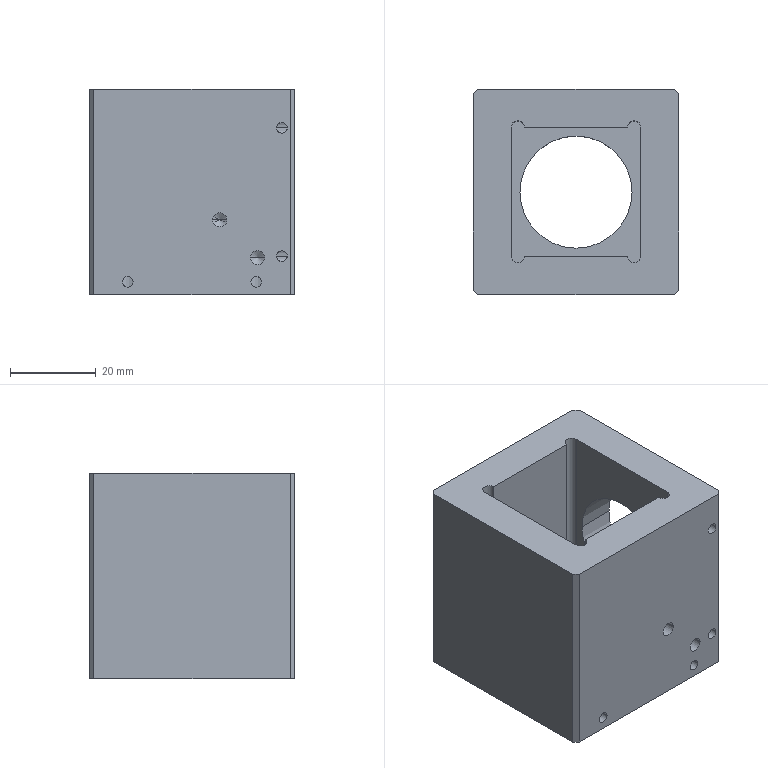NC program | NX | posted with a generic post | part box 48 x 48 x 48 mm
Lines 2794 to 3850 of 9644:
(ZLEVEL_PROFILE_1 , TOOL : D6)
N5562 T12 M6
N5564 G54
N5566 G17 G0 G90 X9.054 Y-10.9 B0. C0. S9500 M3
N5568 G43 Z30. H12
N5570 Z-0.5
N5572 G94 G1 X9.574 Y-11.8 F1000.
N5574 G3 X10.094 Y-12.1 R0.6
N5576 G1 X12.1
N5578 Y-10.094
N5580 G3 X11.8 Y-9.574 R0.6
N5582 G1 X10.9 Y-9.054
N5584 G0 X9.054 Y-10.9 Z-1.
N5586 G1 X9.574 Y-11.8
N5588 G3 X10.094 Y-12.1 R0.6
N5590 G1 X12.1
N5592 Y-10.094
N5594 G3 X11.8 Y-9.574 R0.6
N5596 G1 X10.9 Y-9.054
N5598 G0 X9.054 Y-10.9 Z-1.5
N5600 G1 X9.574 Y-11.8
N5602 G3 X10.094 Y-12.1 R0.6
N5604 G1 X12.1
N5606 Y-10.094
N5608 G3 X11.8 Y-9.574 R0.6
N5610 G1 X10.9 Y-9.054
N5612 G0 X9.054 Y-10.9 Z-2.
N5614 G1 X9.574 Y-11.8
N5616 G3 X10.094 Y-12.1 R0.6
N5618 G1 X12.1
N5620 Y-10.094
N5622 G3 X11.8 Y-9.574 R0.6
N5624 G1 X10.9 Y-9.054
N5626 G0 X9.054 Y-10.9 Z-2.5
N5628 G1 X9.574 Y-11.8
N5630 G3 X10.094 Y-12.1 R0.6
N5632 G1 X12.1
N5634 Y-10.094
N5636 G3 X11.8 Y-9.574 R0.6
N5638 G1 X10.9 Y-9.054
N5640 G0 X9.054 Y-10.9 Z-3.
N5642 G1 X9.574 Y-11.8
N5644 G3 X10.094 Y-12.1 R0.6
N5646 G1 X12.1
N5648 Y-10.094
N5650 G3 X11.8 Y-9.574 R0.6
N5652 G1 X10.9 Y-9.054
N5654 G0 X9.054 Y-10.9 Z-3.5
N5656 G1 X9.574 Y-11.8
N5658 G3 X10.094 Y-12.1 R0.6
N5660 G1 X12.1
N5662 Y-10.094
N5664 G3 X11.8 Y-9.574 R0.6
N5666 G1 X10.9 Y-9.054
N5668 G0 X9.054 Y-10.9 Z-4.
N5670 G1 X9.574 Y-11.8
N5672 G3 X10.094 Y-12.1 R0.6
N5674 G1 X12.1
N5676 Y-10.094
N5678 G3 X11.8 Y-9.574 R0.6
N5680 G1 X10.9 Y-9.054
N5682 G0 X9.054 Y-10.9 Z-4.5
N5684 G1 X9.574 Y-11.8
N5686 G3 X10.094 Y-12.1 R0.6
N5688 G1 X12.1
N5690 Y-10.094
N5692 G3 X11.8 Y-9.574 R0.6
N5694 G1 X10.9 Y-9.054
N5696 G0 X9.054 Y-10.9 Z-5.
N5698 G1 X9.574 Y-11.8
N5700 G3 X10.094 Y-12.1 R0.6
N5702 G1 X12.1
N5704 Y-10.094
N5706 G3 X11.8 Y-9.574 R0.6
N5708 G1 X10.9 Y-9.054
N5710 G0 X9.054 Y-10.9 Z-5.5
N5712 G1 X9.574 Y-11.8
N5714 G3 X10.094 Y-12.1 R0.6
N5716 G1 X12.1
N5718 Y-10.094
N5720 G3 X11.8 Y-9.574 R0.6
N5722 G1 X10.9 Y-9.054
N5724 G0 X9.054 Y-10.9 Z-6.
N5726 G1 X9.574 Y-11.8
N5728 G3 X10.094 Y-12.1 R0.6
N5730 G1 X12.1
N5732 Y-10.094
N5734 G3 X11.8 Y-9.574 R0.6
N5736 G1 X10.9 Y-9.054
N5738 G0 X9.054 Y-10.9 Z-6.5
N5740 G1 X9.574 Y-11.8
N5742 G3 X10.094 Y-12.1 R0.6
N5744 G1 X12.1
N5746 Y-10.094
N5748 G3 X11.8 Y-9.574 R0.6
N5750 G1 X10.9 Y-9.054
N5752 G0 X9.054 Y-10.9 Z-7.
N5754 G1 X9.574 Y-11.8
N5756 G3 X10.094 Y-12.1 R0.6
N5758 G1 X12.1
N5760 Y-10.094
N5762 G3 X11.8 Y-9.574 R0.6
N5764 G1 X10.9 Y-9.054
N5766 G0 X9.054 Y-10.9 Z-7.5
N5768 G1 X9.574 Y-11.8
N5770 G3 X10.094 Y-12.1 R0.6
N5772 G1 X12.1
N5774 Y-10.094
N5776 G3 X11.8 Y-9.574 R0.6
N5778 G1 X10.9 Y-9.054
N5780 G0 X9.054 Y-10.9 Z-8.
N5782 G1 X9.574 Y-11.8
N5784 G3 X10.094 Y-12.1 R0.6
N5786 G1 X12.1
N5788 Y-10.094
N5790 G3 X11.8 Y-9.574 R0.6
N5792 G1 X10.9 Y-9.054
N5794 G0 X9.054 Y-10.9 Z-8.5
N5796 G1 X9.574 Y-11.8
N5798 G3 X10.094 Y-12.1 R0.6
N5800 G1 X12.1
N5802 Y-10.094
N5804 G3 X11.8 Y-9.574 R0.6
N5806 G1 X10.9 Y-9.054
N5808 G0 X9.054 Y-10.9 Z-9.
N5810 G1 X9.574 Y-11.8
N5812 G3 X10.094 Y-12.1 R0.6
N5814 G1 X12.1
N5816 Y-10.094
N5818 G3 X11.8 Y-9.574 R0.6
N5820 G1 X10.9 Y-9.054
N5822 G0 X9.054 Y-10.9 Z-9.5
N5824 G1 X9.574 Y-11.8
N5826 G3 X10.094 Y-12.1 R0.6
N5828 G1 X12.1
N5830 Y-10.094
N5832 G3 X11.8 Y-9.574 R0.6
N5834 G1 X10.9 Y-9.054
N5836 G0 X9.054 Y-10.9 Z-10.
N5838 G1 X9.574 Y-11.8
N5840 G3 X10.094 Y-12.1 R0.6
N5842 G1 X12.1
N5844 Y-10.094
N5846 G3 X11.8 Y-9.574 R0.6
N5848 G1 X10.9 Y-9.054
N5850 G0 X9.054 Y-10.9 Z-10.5
N5852 G1 X9.574 Y-11.8
N5854 G3 X10.094 Y-12.1 R0.6
N5856 G1 X12.1
N5858 Y-10.094
N5860 G3 X11.8 Y-9.574 R0.6
N5862 G1 X10.9 Y-9.054
N5864 G0 X9.054 Y-10.9 Z-11.
N5866 G1 X9.574 Y-11.8
N5868 G3 X10.094 Y-12.1 R0.6
N5870 G1 X12.1
N5872 Y-10.094
N5874 G3 X11.8 Y-9.574 R0.6
N5876 G1 X10.9 Y-9.054
N5878 G0 X9.054 Y-10.9 Z-11.5
N5880 G1 X9.574 Y-11.8
N5882 G3 X10.094 Y-12.1 R0.6
N5884 G1 X12.1
N5886 Y-10.094
N5888 G3 X11.8 Y-9.574 R0.6
N5890 G1 X10.9 Y-9.054
N5892 G0 X9.054 Y-10.9 Z-12.
N5894 G1 X9.574 Y-11.8
N5896 G3 X10.094 Y-12.1 R0.6
N5898 G1 X12.1
N5900 Y-10.094
N5902 G3 X11.8 Y-9.574 R0.6
N5904 G1 X10.9 Y-9.054
N5906 G0 X9.054 Y-10.9 Z-12.5
N5908 G1 X9.574 Y-11.8
N5910 G3 X10.094 Y-12.1 R0.6
N5912 G1 X12.1
N5914 Y-10.094
N5916 G3 X11.8 Y-9.574 R0.6
N5918 G1 X10.9 Y-9.054
N5920 G0 X9.054 Y-10.9 Z-13.
N5922 G1 X9.574 Y-11.8
N5924 G3 X10.094 Y-12.1 R0.6
N5926 G1 X12.1
N5928 Y-10.094
N5930 G3 X11.8 Y-9.574 R0.6
N5932 G1 X10.9 Y-9.054
N5934 G0 X9.054 Y-10.9 Z-13.5
N5936 G1 X9.574 Y-11.8
N5938 G3 X10.094 Y-12.1 R0.6
N5940 G1 X12.1
N5942 Y-10.094
N5944 G3 X11.8 Y-9.574 R0.6
N5946 G1 X10.9 Y-9.054
N5948 G0 X9.054 Y-10.9 Z-14.
N5950 G1 X9.574 Y-11.8
N5952 G3 X10.094 Y-12.1 R0.6
N5954 G1 X12.1
N5956 Y-10.094
N5958 G3 X11.8 Y-9.574 R0.6
N5960 G1 X10.9 Y-9.054
N5962 G0 X9.054 Y-10.9 Z-14.5
N5964 G1 X9.574 Y-11.8
N5966 G3 X10.094 Y-12.1 R0.6
N5968 G1 X12.1
N5970 Y-10.094
N5972 G3 X11.8 Y-9.574 R0.6
N5974 G1 X10.9 Y-9.054
N5976 G0 X9.054 Y-10.9 Z-15.
N5978 G1 X9.574 Y-11.8
N5980 G3 X10.094 Y-12.1 R0.6
N5982 G1 X12.1
N5984 Y-10.094
N5986 G3 X11.8 Y-9.574 R0.6
N5988 G1 X10.9 Y-9.054
N5990 G0 X9.054 Y-10.9 Z-15.5
N5992 G1 X9.574 Y-11.8
N5994 G3 X10.094 Y-12.1 R0.6
N5996 G1 X12.1
N5998 Y-10.094
N6000 G3 X11.8 Y-9.574 R0.6
N6002 G1 X10.9 Y-9.054
N6004 G0 X9.054 Y-10.9 Z-16.
N6006 G1 X9.574 Y-11.8
N6008 G3 X10.094 Y-12.1 R0.6
N6010 G1 X12.1
N6012 Y-10.094
N6014 G3 X11.8 Y-9.574 R0.6
N6016 G1 X10.9 Y-9.054
N6018 G0 X9.054 Y-10.9 Z-16.5
N6020 G1 X9.574 Y-11.8
N6022 G3 X10.094 Y-12.1 R0.6
N6024 G1 X12.1
N6026 Y-10.094
N6028 G3 X11.8 Y-9.574 R0.6
N6030 G1 X10.9 Y-9.054
N6032 G0 X9.054 Y-10.9 Z-17.
N6034 G1 X9.574 Y-11.8
N6036 G3 X10.094 Y-12.1 R0.6
N6038 G1 X12.1
N6040 Y-10.094
N6042 G3 X11.8 Y-9.574 R0.6
N6044 G1 X10.9 Y-9.054
N6046 G0 X9.054 Y-10.9 Z-17.5
N6048 G1 X9.574 Y-11.8
N6050 G3 X10.094 Y-12.1 R0.6
N6052 G1 X12.1
N6054 Y-10.094
N6056 G3 X11.8 Y-9.574 R0.6
N6058 G1 X10.9 Y-9.054
N6060 G0 X9.054 Y-10.9 Z-18.
N6062 G1 X9.574 Y-11.8
N6064 G3 X10.094 Y-12.1 R0.6
N6066 G1 X12.1
N6068 Y-10.094
N6070 G3 X11.8 Y-9.574 R0.6
N6072 G1 X10.9 Y-9.054
N6074 G0 X9.054 Y-10.9 Z-18.5
N6076 G1 X9.574 Y-11.8
N6078 G3 X10.094 Y-12.1 R0.6
N6080 G1 X12.1
N6082 Y-10.094
N6084 G3 X11.8 Y-9.574 R0.6
N6086 G1 X10.9 Y-9.054
N6088 G0 X9.054 Y-10.9 Z-19.
N6090 G1 X9.574 Y-11.8
N6092 G3 X10.094 Y-12.1 R0.6
N6094 G1 X12.1
N6096 Y-10.094
N6098 G3 X11.8 Y-9.574 R0.6
N6100 G1 X10.9 Y-9.054
N6102 G0 X9.054 Y-10.9 Z-19.5
N6104 G1 X9.574 Y-11.8
N6106 G3 X10.094 Y-12.1 R0.6
N6108 G1 X12.1
N6110 Y-10.094
N6112 G3 X11.8 Y-9.574 R0.6
N6114 G1 X10.9 Y-9.054
N6116 G0 X9.054 Y-10.9 Z-20.
N6118 G1 X9.574 Y-11.8
N6120 G3 X10.094 Y-12.1 R0.6
N6122 G1 X12.1
N6124 Y-10.094
N6126 G3 X11.8 Y-9.574 R0.6
N6128 G1 X10.9 Y-9.054
N6130 G0 X9.054 Y-10.9 Z-20.5
N6132 G1 X9.574 Y-11.8
N6134 G3 X10.094 Y-12.1 R0.6
N6136 G1 X12.1
N6138 Y-10.094
N6140 G3 X11.8 Y-9.574 R0.6
N6142 G1 X10.9 Y-9.054
N6144 G0 X9.054 Y-10.9 Z-21.
N6146 G1 X9.574 Y-11.8
N6148 G3 X10.094 Y-12.1 R0.6
N6150 G1 X12.1
N6152 Y-10.094
N6154 G3 X11.8 Y-9.574 R0.6
N6156 G1 X10.9 Y-9.054
N6158 G0 X9.054 Y-10.9 Z-21.5
N6160 G1 X9.574 Y-11.8
N6162 G3 X10.094 Y-12.1 R0.6
N6164 G1 X12.1
N6166 Y-10.094
N6168 G3 X11.8 Y-9.574 R0.6
N6170 G1 X10.9 Y-9.054
N6172 G0 X9.054 Y-10.9 Z-22.
N6174 G1 X9.574 Y-11.8
N6176 G3 X10.094 Y-12.1 R0.6
N6178 G1 X12.1
N6180 Y-10.094
N6182 G3 X11.8 Y-9.574 R0.6
N6184 G1 X10.9 Y-9.054
N6186 G0 X9.054 Y-10.9 Z-22.5
N6188 G1 X9.574 Y-11.8
N6190 G3 X10.094 Y-12.1 R0.6
N6192 G1 X12.1
N6194 Y-10.094
N6196 G3 X11.8 Y-9.574 R0.6
N6198 G1 X10.9 Y-9.054
N6200 G0 X9.054 Y-10.9 Z-23.
N6202 G1 X9.574 Y-11.8
N6204 G3 X10.094 Y-12.1 R0.6
N6206 G1 X12.1
N6208 Y-10.094
N6210 G3 X11.8 Y-9.574 R0.6
N6212 G1 X10.9 Y-9.054
N6214 G0 X9.054 Y-10.9 Z-23.5
N6216 G1 X9.574 Y-11.8
N6218 G3 X10.094 Y-12.1 R0.6
N6220 G1 X12.1
N6222 Y-10.094
N6224 G3 X11.8 Y-9.574 R0.6
N6226 G1 X10.9 Y-9.054
N6228 G0 X9.054 Y-10.9 Z-24.
N6230 G1 X9.574 Y-11.8
N6232 G3 X10.094 Y-12.1 R0.6
N6234 G1 X12.1
N6236 Y-10.094
N6238 G3 X11.8 Y-9.574 R0.6
N6240 G1 X10.9 Y-9.054
N6242 G0 X9.054 Y-10.9 Z-24.5
N6244 G1 X9.574 Y-11.8
N6246 G3 X10.094 Y-12.1 R0.6
N6248 G1 X12.1
N6250 Y-10.094
N6252 G3 X11.8 Y-9.574 R0.6
N6254 G1 X10.9 Y-9.054
N6256 G0 X9.054 Y-10.9 Z-25.
N6258 G1 X9.574 Y-11.8
N6260 G3 X10.094 Y-12.1 R0.6
N6262 G1 X12.1
N6264 Y-10.094
N6266 G3 X11.8 Y-9.574 R0.6
N6268 G1 X10.9 Y-9.054
N6270 G0 X9.054 Y-10.9 Z-25.5
N6272 G1 X9.574 Y-11.8
N6274 G3 X10.094 Y-12.1 R0.6
N6276 G1 X12.1
N6278 Y-10.094
N6280 G3 X11.8 Y-9.574 R0.6
N6282 G1 X10.9 Y-9.054
N6284 G0 X9.054 Y-10.9 Z-26.
N6286 G1 X9.574 Y-11.8
N6288 G3 X10.094 Y-12.1 R0.6
N6290 G1 X12.1
N6292 Y-10.094
N6294 G3 X11.8 Y-9.574 R0.6
N6296 G1 X10.9 Y-9.054
N6298 G0 X9.054 Y-10.9 Z-26.5
N6300 G1 X9.574 Y-11.8
N6302 G3 X10.094 Y-12.1 R0.6
N6304 G1 X12.1
N6306 Y-10.094
N6308 G3 X11.8 Y-9.574 R0.6
N6310 G1 X10.9 Y-9.054
N6312 G0 X9.054 Y-10.9 Z-27.
N6314 G1 X9.574 Y-11.8
N6316 G3 X10.094 Y-12.1 R0.6
N6318 G1 X12.1
N6320 Y-10.094
N6322 G3 X11.8 Y-9.574 R0.6
N6324 G1 X10.9 Y-9.054
N6326 G0 X9.054 Y-10.9 Z-27.5
N6328 G1 X9.574 Y-11.8
N6330 G3 X10.094 Y-12.1 R0.6
N6332 G1 X12.1
N6334 Y-10.094
N6336 G3 X11.8 Y-9.574 R0.6
N6338 G1 X10.9 Y-9.054
N6340 G0 X9.054 Y-10.9 Z-28.
N6342 G1 X9.574 Y-11.8
N6344 G3 X10.094 Y-12.1 R0.6
N6346 G1 X12.1
N6348 Y-10.094
N6350 G3 X11.8 Y-9.574 R0.6
N6352 G1 X10.9 Y-9.054
N6354 G0 X9.054 Y-10.9 Z-28.5
N6356 G1 X9.574 Y-11.8
N6358 G3 X10.094 Y-12.1 R0.6
N6360 G1 X12.1
N6362 Y-10.094
N6364 G3 X11.8 Y-9.574 R0.6
N6366 G1 X10.9 Y-9.054
N6368 G0 X9.054 Y-10.9 Z-29.
N6370 G1 X9.574 Y-11.8
N6372 G3 X10.094 Y-12.1 R0.6
N6374 G1 X12.1
N6376 Y-10.094
N6378 G3 X11.8 Y-9.574 R0.6
N6380 G1 X10.9 Y-9.054
N6382 G0 X9.054 Y-10.9 Z-29.5
N6384 G1 X9.574 Y-11.8
N6386 G3 X10.094 Y-12.1 R0.6
N6388 G1 X12.1
N6390 Y-10.094
N6392 G3 X11.8 Y-9.574 R0.6
N6394 G1 X10.9 Y-9.054
N6396 G0 X9.054 Y-10.9 Z-30.
N6398 G1 X9.574 Y-11.8
N6400 G3 X10.094 Y-12.1 R0.6
N6402 G1 X12.1
N6404 Y-10.094
N6406 G3 X11.8 Y-9.574 R0.6
N6408 G1 X10.9 Y-9.054
N6410 G0 X9.054 Y-10.9 Z-30.5
N6412 G1 X9.574 Y-11.8
N6414 G3 X10.094 Y-12.1 R0.6
N6416 G1 X12.1
N6418 Y-10.094
N6420 G3 X11.8 Y-9.574 R0.6
N6422 G1 X10.9 Y-9.054
N6424 G0 X9.054 Y-10.9 Z-31.
N6426 G1 X9.574 Y-11.8
N6428 G3 X10.094 Y-12.1 R0.6
N6430 G1 X12.1
N6432 Y-10.094
N6434 G3 X11.8 Y-9.574 R0.6
N6436 G1 X10.9 Y-9.054
N6438 G0 X9.054 Y-10.9 Z-31.5
N6440 G1 X9.574 Y-11.8
N6442 G3 X10.094 Y-12.1 R0.6
N6444 G1 X12.1
N6446 Y-10.094
N6448 G3 X11.8 Y-9.574 R0.6
N6450 G1 X10.9 Y-9.054
N6452 G0 X9.054 Y-10.9 Z-32.
N6454 G1 X9.574 Y-11.8
N6456 G3 X10.094 Y-12.1 R0.6
N6458 G1 X12.1
N6460 Y-10.094
N6462 G3 X11.8 Y-9.574 R0.6
N6464 G1 X10.9 Y-9.054
N6466 G0 X9.054 Y-10.9 Z-32.5
N6468 G1 X9.574 Y-11.8
N6470 G3 X10.094 Y-12.1 R0.6
N6472 G1 X12.1
N6474 Y-10.094
N6476 G3 X11.8 Y-9.574 R0.6
N6478 G1 X10.9 Y-9.054
N6480 G0 X9.054 Y-10.9 Z-33.
N6482 G1 X9.574 Y-11.8
N6484 G3 X10.094 Y-12.1 R0.6
N6486 G1 X12.1
N6488 Y-10.094
N6490 G3 X11.8 Y-9.574 R0.6
N6492 G1 X10.9 Y-9.054
N6494 G0 X9.054 Y-10.9 Z-33.5
N6496 G1 X9.574 Y-11.8
N6498 G3 X10.094 Y-12.1 R0.6
N6500 G1 X12.1
N6502 Y-10.094
N6504 G3 X11.8 Y-9.574 R0.6
N6506 G1 X10.9 Y-9.054
N6508 G0 X9.054 Y-10.9 Z-34.
N6510 G1 X9.574 Y-11.8
N6512 G3 X10.094 Y-12.1 R0.6
N6514 G1 X12.1
N6516 Y-10.094
N6518 G3 X11.8 Y-9.574 R0.6
N6520 G1 X10.9 Y-9.054
N6522 G0 X9.054 Y-10.9 Z-34.5
N6524 G1 X9.574 Y-11.8
N6526 G3 X10.094 Y-12.1 R0.6
N6528 G1 X12.1
N6530 Y-10.094
N6532 G3 X11.8 Y-9.574 R0.6
N6534 G1 X10.9 Y-9.054
N6536 G0 X9.054 Y-10.9 Z-35.
N6538 G1 X9.574 Y-11.8
N6540 G3 X10.094 Y-12.1 R0.6
N6542 G1 X12.1
N6544 Y-10.094
N6546 G3 X11.8 Y-9.574 R0.6
N6548 G1 X10.9 Y-9.054
N6550 G0 X9.054 Y-10.9 Z-35.5
N6552 G1 X9.574 Y-11.8
N6554 G3 X10.094 Y-12.1 R0.6
N6556 G1 X12.1
N6558 Y-10.094
N6560 G3 X11.8 Y-9.574 R0.6
N6562 G1 X10.9 Y-9.054
N6564 G0 X9.054 Y-10.9 Z-36.
N6566 G1 X9.574 Y-11.8
N6568 G3 X10.094 Y-12.1 R0.6
N6570 G1 X12.1
N6572 Y-10.094
N6574 G3 X11.8 Y-9.574 R0.6
N6576 G1 X10.9 Y-9.054
N6578 G0 X9.054 Y-10.9 Z-36.5
N6580 G1 X9.574 Y-11.8
N6582 G3 X10.094 Y-12.1 R0.6
N6584 G1 X12.1
N6586 Y-10.094
N6588 G3 X11.8 Y-9.574 R0.6
N6590 G1 X10.9 Y-9.054
N6592 G0 X9.054 Y-10.9 Z-37.
N6594 G1 X9.574 Y-11.8
N6596 G3 X10.094 Y-12.1 R0.6
N6598 G1 X12.1
N6600 Y-10.094
N6602 G3 X11.8 Y-9.574 R0.6
N6604 G1 X10.9 Y-9.054
N6606 G0 X9.054 Y-10.9 Z-37.5
N6608 G1 X9.574 Y-11.8
N6610 G3 X10.094 Y-12.1 R0.6
N6612 G1 X12.1
N6614 Y-10.094
N6616 G3 X11.8 Y-9.574 R0.6
N6618 G1 X10.9 Y-9.054
N6620 G0 X9.054 Y-10.9 Z-38.
N6622 G1 X9.574 Y-11.8
N6624 G3 X10.094 Y-12.1 R0.6
N6626 G1 X12.1
N6628 Y-10.094
N6630 G3 X11.8 Y-9.574 R0.6
N6632 G1 X10.9 Y-9.054
N6634 G0 X9.054 Y-10.9 Z-38.5
N6636 G1 X9.574 Y-11.8
N6638 G3 X10.094 Y-12.1 R0.6
N6640 G1 X12.1
N6642 Y-10.094
N6644 G3 X11.8 Y-9.574 R0.6
N6646 G1 X10.9 Y-9.054
N6648 G0 X9.054 Y-10.9 Z-39.
N6650 G1 X9.574 Y-11.8
N6652 G3 X10.094 Y-12.1 R0.6
N6654 G1 X12.1
N6656 Y-10.094
N6658 G3 X11.8 Y-9.574 R0.6
N6660 G1 X10.9 Y-9.054
N6662 G0 Z30.
N6664 Y9.054
N6666 Z-0.5
N6668 G1 X11.8 Y9.574
N6670 G3 X12.1 Y10.094 R0.6
N6672 G1 Y12.1
N6674 X10.094
N6676 G3 X9.574 Y11.8 R0.6
N6678 G1 X9.054 Y10.9
N6680 G0 X10.9 Y9.054 Z-1.
N6682 G1 X11.8 Y9.574
N6684 G3 X12.1 Y10.094 R0.6
N6686 G1 Y12.1
N6688 X10.094
N6690 G3 X9.574 Y11.8 R0.6
N6692 G1 X9.054 Y10.9
N6694 G0 X10.9 Y9.054 Z-1.5
N6696 G1 X11.8 Y9.574
N6698 G3 X12.1 Y10.094 R0.6
N6700 G1 Y12.1
N6702 X10.094
N6704 G3 X9.574 Y11.8 R0.6
N6706 G1 X9.054 Y10.9
N6708 G0 X10.9 Y9.054 Z-2.
N6710 G1 X11.8 Y9.574
N6712 G3 X12.1 Y10.094 R0.6
N6714 G1 Y12.1
N6716 X10.094
N6718 G3 X9.574 Y11.8 R0.6
N6720 G1 X9.054 Y10.9
N6722 G0 X10.9 Y9.054 Z-2.5
N6724 G1 X11.8 Y9.574
N6726 G3 X12.1 Y10.094 R0.6
N6728 G1 Y12.1
N6730 X10.094
N6732 G3 X9.574 Y11.8 R0.6
N6734 G1 X9.054 Y10.9
N6736 G0 X10.9 Y9.054 Z-3.
N6738 G1 X11.8 Y9.574
N6740 G3 X12.1 Y10.094 R0.6
N6742 G1 Y12.1
N6744 X10.094
N6746 G3 X9.574 Y11.8 R0.6
N6748 G1 X9.054 Y10.9
N6750 G0 X10.9 Y9.054 Z-3.5
N6752 G1 X11.8 Y9.574
N6754 G3 X12.1 Y10.094 R0.6
N6756 G1 Y12.1
N6758 X10.094
N6760 G3 X9.574 Y11.8 R0.6
N6762 G1 X9.054 Y10.9
N6764 G0 X10.9 Y9.054 Z-4.
N6766 G1 X11.8 Y9.574
N6768 G3 X12.1 Y10.094 R0.6
N6770 G1 Y12.1
N6772 X10.094
N6774 G3 X9.574 Y11.8 R0.6
N6776 G1 X9.054 Y10.9
N6778 G0 X10.9 Y9.054 Z-4.5
N6780 G1 X11.8 Y9.574
N6782 G3 X12.1 Y10.094 R0.6
N6784 G1 Y12.1
N6786 X10.094
N6788 G3 X9.574 Y11.8 R0.6
N6790 G1 X9.054 Y10.9
N6792 G0 X10.9 Y9.054 Z-5.
N6794 G1 X11.8 Y9.574
N6796 G3 X12.1 Y10.094 R0.6
N6798 G1 Y12.1
N6800 X10.094
N6802 G3 X9.574 Y11.8 R0.6
N6804 G1 X9.054 Y10.9
N6806 G0 X10.9 Y9.054 Z-5.5
N6808 G1 X11.8 Y9.574
N6810 G3 X12.1 Y10.094 R0.6
N6812 G1 Y12.1
N6814 X10.094
N6816 G3 X9.574 Y11.8 R0.6
N6818 G1 X9.054 Y10.9
N6820 G0 X10.9 Y9.054 Z-6.
N6822 G1 X11.8 Y9.574
N6824 G3 X12.1 Y10.094 R0.6
N6826 G1 Y12.1
N6828 X10.094
N6830 G3 X9.574 Y11.8 R0.6
N6832 G1 X9.054 Y10.9
N6834 G0 X10.9 Y9.054 Z-6.5
N6836 G1 X11.8 Y9.574
N6838 G3 X12.1 Y10.094 R0.6
N6840 G1 Y12.1
N6842 X10.094
N6844 G3 X9.574 Y11.8 R0.6
N6846 G1 X9.054 Y10.9
N6848 G0 X10.9 Y9.054 Z-7.
N6850 G1 X11.8 Y9.574
N6852 G3 X12.1 Y10.094 R0.6
N6854 G1 Y12.1
N6856 X10.094
N6858 G3 X9.574 Y11.8 R0.6
N6860 G1 X9.054 Y10.9
N6862 G0 X10.9 Y9.054 Z-7.5
N6864 G1 X11.8 Y9.574
N6866 G3 X12.1 Y10.094 R0.6
N6868 G1 Y12.1
N6870 X10.094
N6872 G3 X9.574 Y11.8 R0.6
N6874 G1 X9.054 Y10.9
N6876 G0 X10.9 Y9.054 Z-8.
N6878 G1 X11.8 Y9.574
N6880 G3 X12.1 Y10.094 R0.6
N6882 G1 Y12.1
N6884 X10.094
N6886 G3 X9.574 Y11.8 R0.6
N6888 G1 X9.054 Y10.9
N6890 G0 X10.9 Y9.054 Z-8.5
N6892 G1 X11.8 Y9.574
N6894 G3 X12.1 Y10.094 R0.6
N6896 G1 Y12.1
N6898 X10.094
N6900 G3 X9.574 Y11.8 R0.6
N6902 G1 X9.054 Y10.9
N6904 G0 X10.9 Y9.054 Z-9.
N6906 G1 X11.8 Y9.574
N6908 G3 X12.1 Y10.094 R0.6
N6910 G1 Y12.1
N6912 X10.094
N6914 G3 X9.574 Y11.8 R0.6
N6916 G1 X9.054 Y10.9
N6918 G0 X10.9 Y9.054 Z-9.5
N6920 G1 X11.8 Y9.574
N6922 G3 X12.1 Y10.094 R0.6
N6924 G1 Y12.1
N6926 X10.094
N6928 G3 X9.574 Y11.8 R0.6
N6930 G1 X9.054 Y10.9
N6932 G0 X10.9 Y9.054 Z-10.
N6934 G1 X11.8 Y9.574
N6936 G3 X12.1 Y10.094 R0.6
N6938 G1 Y12.1
N6940 X10.094
N6942 G3 X9.574 Y11.8 R0.6
N6944 G1 X9.054 Y10.9
N6946 G0 X10.9 Y9.054 Z-10.5
N6948 G1 X11.8 Y9.574
N6950 G3 X12.1 Y10.094 R0.6
N6952 G1 Y12.1
N6954 X10.094
N6956 G3 X9.574 Y11.8 R0.6
N6958 G1 X9.054 Y10.9
N6960 G0 X10.9 Y9.054 Z-11.
N6962 G1 X11.8 Y9.574
N6964 G3 X12.1 Y10.094 R0.6
N6966 G1 Y12.1
N6968 X10.094
N6970 G3 X9.574 Y11.8 R0.6
N6972 G1 X9.054 Y10.9
N6974 G0 X10.9 Y9.054 Z-11.5
N6976 G1 X11.8 Y9.574
N6978 G3 X12.1 Y10.094 R0.6
N6980 G1 Y12.1
N6982 X10.094
N6984 G3 X9.574 Y11.8 R0.6
N6986 G1 X9.054 Y10.9
N6988 G0 X10.9 Y9.054 Z-12.
N6990 G1 X11.8 Y9.574
N6992 G3 X12.1 Y10.094 R0.6
N6994 G1 Y12.1
N6996 X10.094
N6998 G3 X9.574 Y11.8 R0.6
N7000 G1 X9.054 Y10.9
N7002 G0 X10.9 Y9.054 Z-12.5
N7004 G1 X11.8 Y9.574
N7006 G3 X12.1 Y10.094 R0.6
N7008 G1 Y12.1
N7010 X10.094
N7012 G3 X9.574 Y11.8 R0.6
N7014 G1 X9.054 Y10.9
N7016 G0 X10.9 Y9.054 Z-13.
N7018 G1 X11.8 Y9.574
N7020 G3 X12.1 Y10.094 R0.6
N7022 G1 Y12.1
N7024 X10.094
N7026 G3 X9.574 Y11.8 R0.6
N7028 G1 X9.054 Y10.9
N7030 G0 X10.9 Y9.054 Z-13.5
N7032 G1 X11.8 Y9.574
N7034 G3 X12.1 Y10.094 R0.6
N7036 G1 Y12.1
N7038 X10.094
N7040 G3 X9.574 Y11.8 R0.6
N7042 G1 X9.054 Y10.9
N7044 G0 X10.9 Y9.054 Z-14.
N7046 G1 X11.8 Y9.574
N7048 G3 X12.1 Y10.094 R0.6
N7050 G1 Y12.1
N7052 X10.094
N7054 G3 X9.574 Y11.8 R0.6
N7056 G1 X9.054 Y10.9
N7058 G0 X10.9 Y9.054 Z-14.5
N7060 G1 X11.8 Y9.574
N7062 G3 X12.1 Y10.094 R0.6
N7064 G1 Y12.1
N7066 X10.094
N7068 G3 X9.574 Y11.8 R0.6
N7070 G1 X9.054 Y10.9
N7072 G0 X10.9 Y9.054 Z-15.
N7074 G1 X11.8 Y9.574
N7076 G3 X12.1 Y10.094 R0.6
N7078 G1 Y12.1
N7080 X10.094
N7082 G3 X9.574 Y11.8 R0.6
N7084 G1 X9.054 Y10.9
N7086 G0 X10.9 Y9.054 Z-15.5
N7088 G1 X11.8 Y9.574
N7090 G3 X12.1 Y10.094 R0.6
N7092 G1 Y12.1
N7094 X10.094
N7096 G3 X9.574 Y11.8 R0.6
N7098 G1 X9.054 Y10.9
N7100 G0 X10.9 Y9.054 Z-16.
N7102 G1 X11.8 Y9.574
N7104 G3 X12.1 Y10.094 R0.6
N7106 G1 Y12.1
N7108 X10.094
N7110 G3 X9.574 Y11.8 R0.6
N7112 G1 X9.054 Y10.9
N7114 G0 X10.9 Y9.054 Z-16.5
N7116 G1 X11.8 Y9.574
N7118 G3 X12.1 Y10.094 R0.6
N7120 G1 Y12.1
N7122 X10.094
N7124 G3 X9.574 Y11.8 R0.6
N7126 G1 X9.054 Y10.9
N7128 G0 X10.9 Y9.054 Z-17.
N7130 G1 X11.8 Y9.574
N7132 G3 X12.1 Y10.094 R0.6
N7134 G1 Y12.1
N7136 X10.094
N7138 G3 X9.574 Y11.8 R0.6
N7140 G1 X9.054 Y10.9
N7142 G0 X10.9 Y9.054 Z-17.5
N7144 G1 X11.8 Y9.574
N7146 G3 X12.1 Y10.094 R0.6
N7148 G1 Y12.1
N7150 X10.094
N7152 G3 X9.574 Y11.8 R0.6
N7154 G1 X9.054 Y10.9
N7156 G0 X10.9 Y9.054 Z-18.
N7158 G1 X11.8 Y9.574
N7160 G3 X12.1 Y10.094 R0.6
N7162 G1 Y12.1
N7164 X10.094
N7166 G3 X9.574 Y11.8 R0.6
N7168 G1 X9.054 Y10.9
N7170 G0 X10.9 Y9.054 Z-18.5
N7172 G1 X11.8 Y9.574
N7174 G3 X12.1 Y10.094 R0.6
N7176 G1 Y12.1
N7178 X10.094
N7180 G3 X9.574 Y11.8 R0.6
N7182 G1 X9.054 Y10.9
N7184 G0 X10.9 Y9.054 Z-19.
N7186 G1 X11.8 Y9.574
N7188 G3 X12.1 Y10.094 R0.6
N7190 G1 Y12.1
N7192 X10.094
N7194 G3 X9.574 Y11.8 R0.6
N7196 G1 X9.054 Y10.9
N7198 G0 X10.9 Y9.054 Z-19.5
N7200 G1 X11.8 Y9.574
N7202 G3 X12.1 Y10.094 R0.6
N7204 G1 Y12.1
N7206 X10.094
N7208 G3 X9.574 Y11.8 R0.6
N7210 G1 X9.054 Y10.9
N7212 G0 X10.9 Y9.054 Z-20.
N7214 G1 X11.8 Y9.574
N7216 G3 X12.1 Y10.094 R0.6
N7218 G1 Y12.1
N7220 X10.094
N7222 G3 X9.574 Y11.8 R0.6
N7224 G1 X9.054 Y10.9
N7226 G0 X10.9 Y9.054 Z-20.5
N7228 G1 X11.8 Y9.574
N7230 G3 X12.1 Y10.094 R0.6
N7232 G1 Y12.1
N7234 X10.094
N7236 G3 X9.574 Y11.8 R0.6
N7238 G1 X9.054 Y10.9
N7240 G0 X10.9 Y9.054 Z-21.
N7242 G1 X11.8 Y9.574
N7244 G3 X12.1 Y10.094 R0.6
N7246 G1 Y12.1
N7248 X10.094
N7250 G3 X9.574 Y11.8 R0.6
N7252 G1 X9.054 Y10.9
N7254 G0 X10.9 Y9.054 Z-21.5
N7256 G1 X11.8 Y9.574
N7258 G3 X12.1 Y10.094 R0.6
N7260 G1 Y12.1
N7262 X10.094
N7264 G3 X9.574 Y11.8 R0.6
N7266 G1 X9.054 Y10.9
N7268 G0 X10.9 Y9.054 Z-22.
N7270 G1 X11.8 Y9.574
N7272 G3 X12.1 Y10.094 R0.6
N7274 G1 Y12.1
N7276 X10.094
N7278 G3 X9.574 Y11.8 R0.6
N7280 G1 X9.054 Y10.9
N7282 G0 X10.9 Y9.054 Z-22.5
N7284 G1 X11.8 Y9.574
N7286 G3 X12.1 Y10.094 R0.6
N7288 G1 Y12.1
N7290 X10.094
N7292 G3 X9.574 Y11.8 R0.6
N7294 G1 X9.054 Y10.9
N7296 G0 X10.9 Y9.054 Z-23.
N7298 G1 X11.8 Y9.574
N7300 G3 X12.1 Y10.094 R0.6
N7302 G1 Y12.1
N7304 X10.094
N7306 G3 X9.574 Y11.8 R0.6
N7308 G1 X9.054 Y10.9
N7310 G0 X10.9 Y9.054 Z-23.5
N7312 G1 X11.8 Y9.574
N7314 G3 X12.1 Y10.094 R0.6
N7316 G1 Y12.1
N7318 X10.094
N7320 G3 X9.574 Y11.8 R0.6
N7322 G1 X9.054 Y10.9
N7324 G0 X10.9 Y9.054 Z-24.
N7326 G1 X11.8 Y9.574
N7328 G3 X12.1 Y10.094 R0.6
N7330 G1 Y12.1
N7332 X10.094
N7334 G3 X9.574 Y11.8 R0.6
N7336 G1 X9.054 Y10.9
N7338 G0 X10.9 Y9.054 Z-24.5
N7340 G1 X11.8 Y9.574
N7342 G3 X12.1 Y10.094 R0.6
N7344 G1 Y12.1
N7346 X10.094
N7348 G3 X9.574 Y11.8 R0.6
N7350 G1 X9.054 Y10.9
N7352 G0 X10.9 Y9.054 Z-25.
N7354 G1 X11.8 Y9.574
N7356 G3 X12.1 Y10.094 R0.6
N7358 G1 Y12.1
N7360 X10.094
N7362 G3 X9.574 Y11.8 R0.6
N7364 G1 X9.054 Y10.9
N7366 G0 X10.9 Y9.054 Z-25.5
N7368 G1 X11.8 Y9.574
N7370 G3 X12.1 Y10.094 R0.6
N7372 G1 Y12.1
N7374 X10.094
N7376 G3 X9.574 Y11.8 R0.6
N7378 G1 X9.054 Y10.9
N7380 G0 X10.9 Y9.054 Z-26.
N7382 G1 X11.8 Y9.574
N7384 G3 X12.1 Y10.094 R0.6
N7386 G1 Y12.1
N7388 X10.094
N7390 G3 X9.574 Y11.8 R0.6
N7392 G1 X9.054 Y10.9
N7394 G0 X10.9 Y9.054 Z-26.5
N7396 G1 X11.8 Y9.574
N7398 G3 X12.1 Y10.094 R0.6
N7400 G1 Y12.1
N7402 X10.094
N7404 G3 X9.574 Y11.8 R0.6
N7406 G1 X9.054 Y10.9
N7408 G0 X10.9 Y9.054 Z-27.
N7410 G1 X11.8 Y9.574
N7412 G3 X12.1 Y10.094 R0.6
N7414 G1 Y12.1
N7416 X10.094
N7418 G3 X9.574 Y11.8 R0.6
N7420 G1 X9.054 Y10.9
N7422 G0 X10.9 Y9.054 Z-27.5
N7424 G1 X11.8 Y9.574
N7426 G3 X12.1 Y10.094 R0.6
N7428 G1 Y12.1
N7430 X10.094
N7432 G3 X9.574 Y11.8 R0.6
N7434 G1 X9.054 Y10.9
N7436 G0 X10.9 Y9.054 Z-28.
N7438 G1 X11.8 Y9.574
N7440 G3 X12.1 Y10.094 R0.6
N7442 G1 Y12.1
N7444 X10.094
N7446 G3 X9.574 Y11.8 R0.6
N7448 G1 X9.054 Y10.9
N7450 G0 X10.9 Y9.054 Z-28.5
N7452 G1 X11.8 Y9.574
N7454 G3 X12.1 Y10.094 R0.6
N7456 G1 Y12.1
N7458 X10.094
N7460 G3 X9.574 Y11.8 R0.6
N7462 G1 X9.054 Y10.9
N7464 G0 X10.9 Y9.054 Z-29.
N7466 G1 X11.8 Y9.574
N7468 G3 X12.1 Y10.094 R0.6
N7470 G1 Y12.1
N7472 X10.094
N7474 G3 X9.574 Y11.8 R0.6
N7476 G1 X9.054 Y10.9
N7478 G0 X10.9 Y9.054 Z-29.5
N7480 G1 X11.8 Y9.574
N7482 G3 X12.1 Y10.094 R0.6
N7484 G1 Y12.1
N7486 X10.094
N7488 G3 X9.574 Y11.8 R0.6
N7490 G1 X9.054 Y10.9
N7492 G0 X10.9 Y9.054 Z-30.
N7494 G1 X11.8 Y9.574
N7496 G3 X12.1 Y10.094 R0.6
N7498 G1 Y12.1
N7500 X10.094
N7502 G3 X9.574 Y11.8 R0.6
N7504 G1 X9.054 Y10.9
N7506 G0 X10.9 Y9.054 Z-30.5
N7508 G1 X11.8 Y9.574
N7510 G3 X12.1 Y10.094 R0.6
N7512 G1 Y12.1
N7514 X10.094
N7516 G3 X9.574 Y11.8 R0.6
N7518 G1 X9.054 Y10.9
N7520 G0 X10.9 Y9.054 Z-31.
N7522 G1 X11.8 Y9.574
N7524 G3 X12.1 Y10.094 R0.6
N7526 G1 Y12.1
N7528 X10.094
N7530 G3 X9.574 Y11.8 R0.6
N7532 G1 X9.054 Y10.9
N7534 G0 X10.9 Y9.054 Z-31.5
N7536 G1 X11.8 Y9.574
N7538 G3 X12.1 Y10.094 R0.6
N7540 G1 Y12.1
N7542 X10.094
N7544 G3 X9.574 Y11.8 R0.6
N7546 G1 X9.054 Y10.9
N7548 G0 X10.9 Y9.054 Z-32.
N7550 G1 X11.8 Y9.574
N7552 G3 X12.1 Y10.094 R0.6
N7554 G1 Y12.1
N7556 X10.094
N7558 G3 X9.574 Y11.8 R0.6
N7560 G1 X9.054 Y10.9
N7562 G0 X10.9 Y9.054 Z-32.5
N7564 G1 X11.8 Y9.574
N7566 G3 X12.1 Y10.094 R0.6
N7568 G1 Y12.1
N7570 X10.094
N7572 G3 X9.574 Y11.8 R0.6
N7574 G1 X9.054 Y10.9
N7576 G0 X10.9 Y9.054 Z-33.
N7578 G1 X11.8 Y9.574
N7580 G3 X12.1 Y10.094 R0.6
N7582 G1 Y12.1
N7584 X10.094
N7586 G3 X9.574 Y11.8 R0.6
N7588 G1 X9.054 Y10.9
N7590 G0 X10.9 Y9.054 Z-33.5
N7592 G1 X11.8 Y9.574
N7594 G3 X12.1 Y10.094 R0.6
N7596 G1 Y12.1
N7598 X10.094
N7600 G3 X9.574 Y11.8 R0.6
N7602 G1 X9.054 Y10.9
N7604 G0 X10.9 Y9.054 Z-34.
N7606 G1 X11.8 Y9.574
N7608 G3 X12.1 Y10.094 R0.6
N7610 G1 Y12.1
N7612 X10.094
N7614 G3 X9.574 Y11.8 R0.6
N7616 G1 X9.054 Y10.9
N7618 G0 X10.9 Y9.054 Z-34.5
N7620 G1 X11.8 Y9.574
N7622 G3 X12.1 Y10.094 R0.6
N7624 G1 Y12.1
N7626 X10.094
N7628 G3 X9.574 Y11.8 R0.6
N7630 G1 X9.054 Y10.9
N7632 G0 X10.9 Y9.054 Z-35.
N7634 G1 X11.8 Y9.574
N7636 G3 X12.1 Y10.094 R0.6
N7638 G1 Y12.1
N7640 X10.094
N7642 G3 X9.574 Y11.8 R0.6
N7644 G1 X9.054 Y10.9
N7646 G0 X10.9 Y9.054 Z-35.5
N7648 G1 X11.8 Y9.574
N7650 G3 X12.1 Y10.094 R0.6
N7652 G1 Y12.1
N7654 X10.094
N7656 G3 X9.574 Y11.8 R0.6
N7658 G1 X9.054 Y10.9
N7660 G0 X10.9 Y9.054 Z-36.
N7662 G1 X11.8 Y9.574
N7664 G3 X12.1 Y10.094 R0.6
N7666 G1 Y12.1
N7668 X10.094